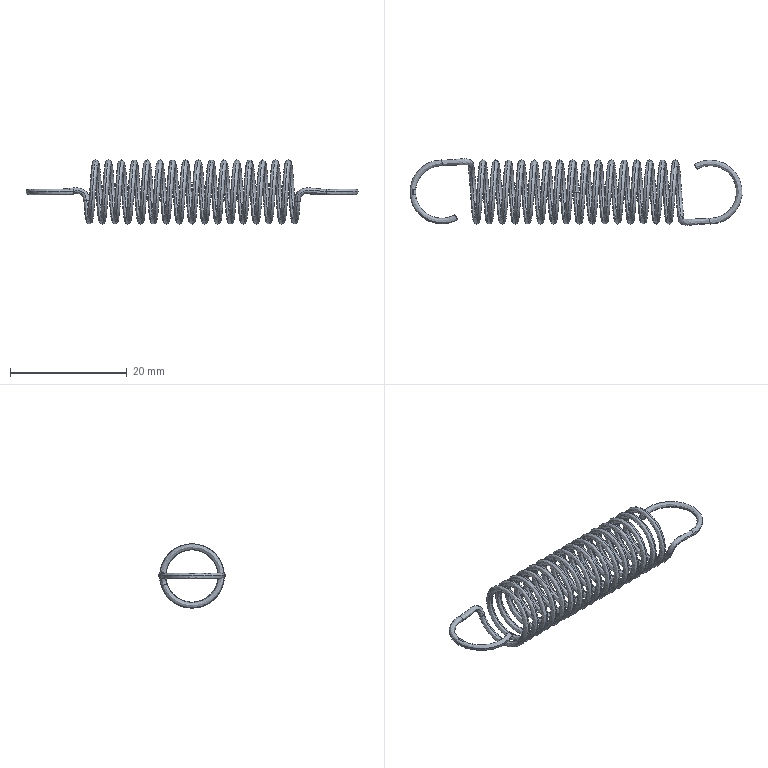Part | SolidWorks | features 3DProfileFeature 2, CirPattern 1, CombineBodies 1, Helix 1, ICE 1, Sweep 1 | 1 solid | 19 faces | box 56.999 x 11.387 x 10.999 mm | volume 441.954 mm3 | spline 12 | plane 4 | cylinder 3 | commonest cylinder face diameters 1 x3